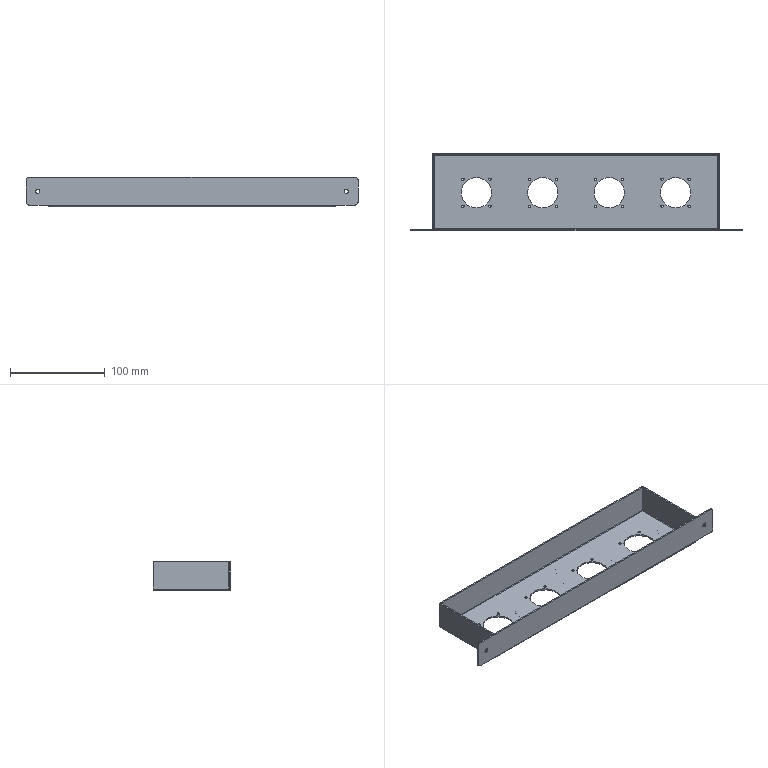Part | STEP file | interface connection plate | 1 solid | 449 faces | box 350 x 81.5 x 31.5 mm | volume 67618 mm3 | plane 227 | spline 166 | cylinder 56 | commonest cylinder face diameters 2.5 x32 32 x8 1 x4 4 x4 4.5 x4 6 x4